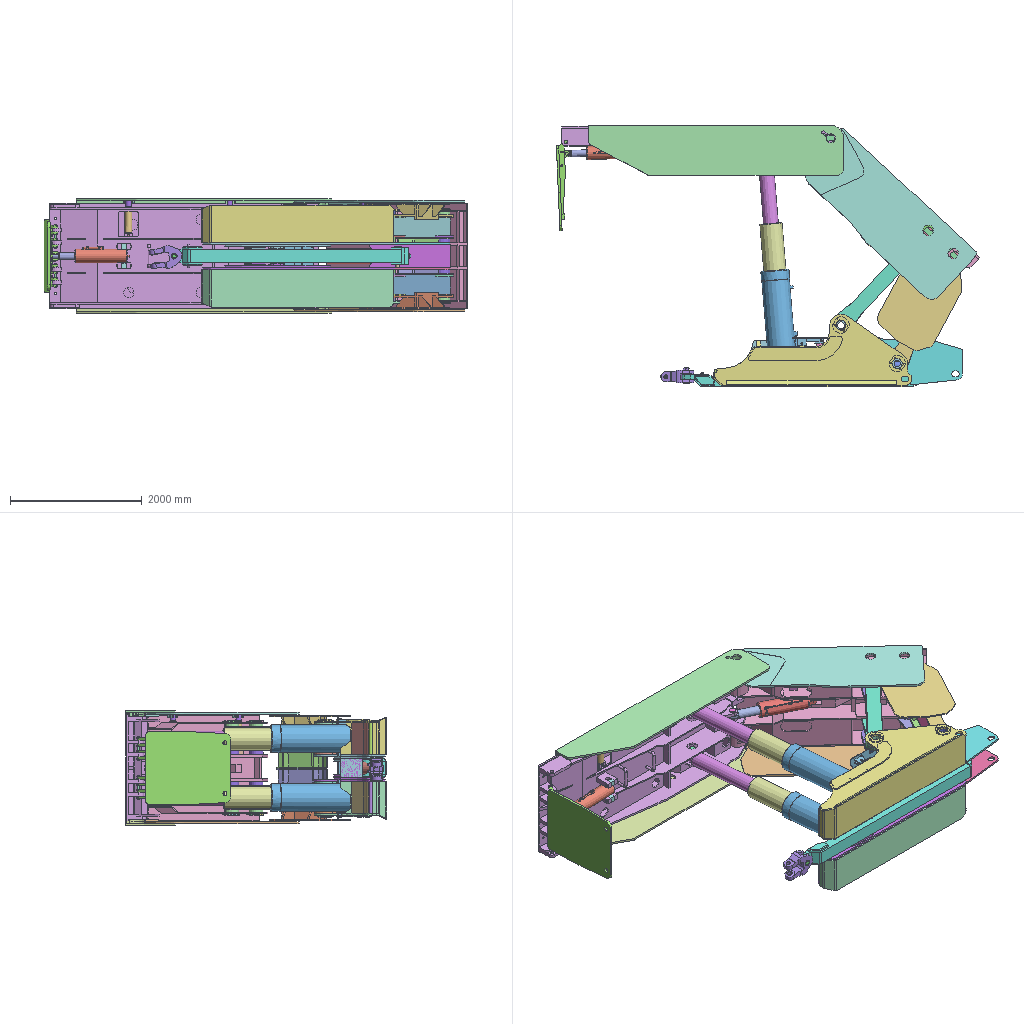Assembly | NX | 121 different items | 178 placed | box 6418 x 3966 x 1741 mm
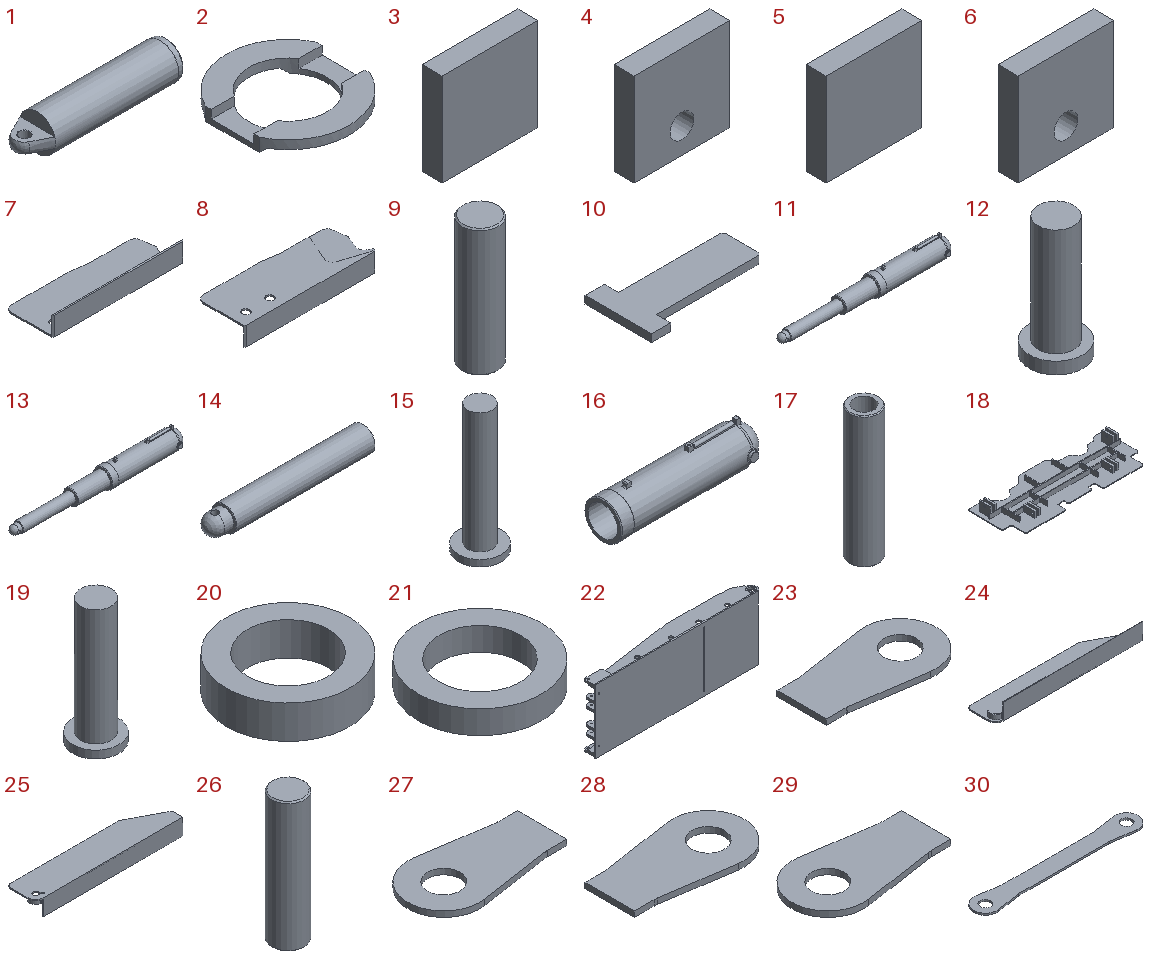Parts list (item | quantity | parent item | size | volume | features):
1 | x4 | in 56, 67, 78, 89 | 448 x 106 x 106 mm | 2799935 mm3 | features 侧推千斤顶缸 2
2 | x1 | in 34 | 207.123 x 230 x 25 mm | 362169 mm3 | features 掩护梁 2
3 | x1 | in 34 | 120 x 25 x 116 mm | 333863 mm3 | features 掩护梁 2
4 | x1 | in 34 | 120 x 25 x 116 mm | 330329 mm3 | features 掩护梁 2
5 | x1 | in 34 | 120 x 25 x 116 mm | 333863 mm3 | features 掩护梁 2
6 | x1 | in 34 | 120 x 25 x 116 mm | 330329 mm3 | features 掩护梁 2
7 | x1 | in 34 | 2828 x 1030 x 405 mm | 109386503 mm3 | features 掩护梁侧护板右 2
8 | x1 | in 34 | 2828 x 1030 x 405 mm | 109946345 mm3 | features 掩护梁侧护板左 2
9 | x4 | - | 145 x 145 x 511 mm | 8427015 mm3 | features 掩护梁连杆柱销 2
10 | x6 | in 34 | 260 x 140 x 16 mm | 370800 mm3 | features 梁销挡板 2
11 | x1 | - | 3742 x 478 x 474 mm | 232387520 mm3 | features 立柱活塞 2, 立柱缸一级 2, 立柱缸二级 2
12 | x4 | in 34 | 45 x 45 x 100 mm | 79522 mm3 | features 侧推千斤顶缸销 2
13 | x1 | - | 3742 x 478 x 474 mm | 232387520 mm3 | features 立柱活塞 2, 立柱缸一级 2, 立柱缸二级 2
14 | x2 | in 11, 13 | 1466 x 228.3 x 228.3 mm | 56225890 mm3 | features 立柱活塞 2
15 | x2 | - | 100 x 100 x 295 mm | 832302 mm3 | features 立柱活塞销 2
16 | x2 | in 11, 13 | 1697 x 478 x 474 mm | 93646895 mm3 | features 立柱缸一级 2
17 | x2 | in 11, 13 | 337.48 x 337.48 x 1508 mm | 82514797 mm3 | features 立柱缸二级 2
18 | x1 | in 45 | 1560 x 608.47 x 118 mm | 9927777 mm3 | features 脚踏板 2
19 | x4 | in 45 | 30 x 30 x 81 mm | 27410 mm3 | features 脚踏板柱销 2
20 | x4 | - | 220 x 220 x 59.435 mm | 1277869 mm3 | features 连杆套筒内 2
21 | x4 | - | 220 x 220 x 41.57 mm | 893766 mm3 | features 连杆套筒外 2
22 | x1 | in 34 | 4215 x 507.464 x 1600 mm | 647411376 mm3 | features 顶梁 2
23 | x2 | in 45 | 597.539 x 319.958 x 25 mm | 3444700 mm3 | features 前连杆 2
24 | x1 | in 34 | 3880 x 760 x 430 mm | 99045232 mm3 | features 顶梁侧护板右 2
25 | x1 | in 34 | 3880 x 760 x 430 mm | 99665785 mm3 | features 顶梁侧护板左 2
26 | x2 | in 34 | 130 x 130 x 520 mm | 6892131 mm3 | features 顶梁掩护板柱销 2
27 | x2 | in 45 | 597.539 x 319.958 x 25 mm | 3444700 mm3 | features 前连杆 2
28 | x2 | in 45 | 597.7 x 320 x 25 mm | 3443870 mm3 | features 前连杆 2
29 | x2 | in 45 | 597.7 x 320 x 25 mm | 3443870 mm3 | features 前连杆 2
30 | x2 | in 45 | 2260 x 320 x 25 mm | 12756678 mm3 | features 前连杆 2
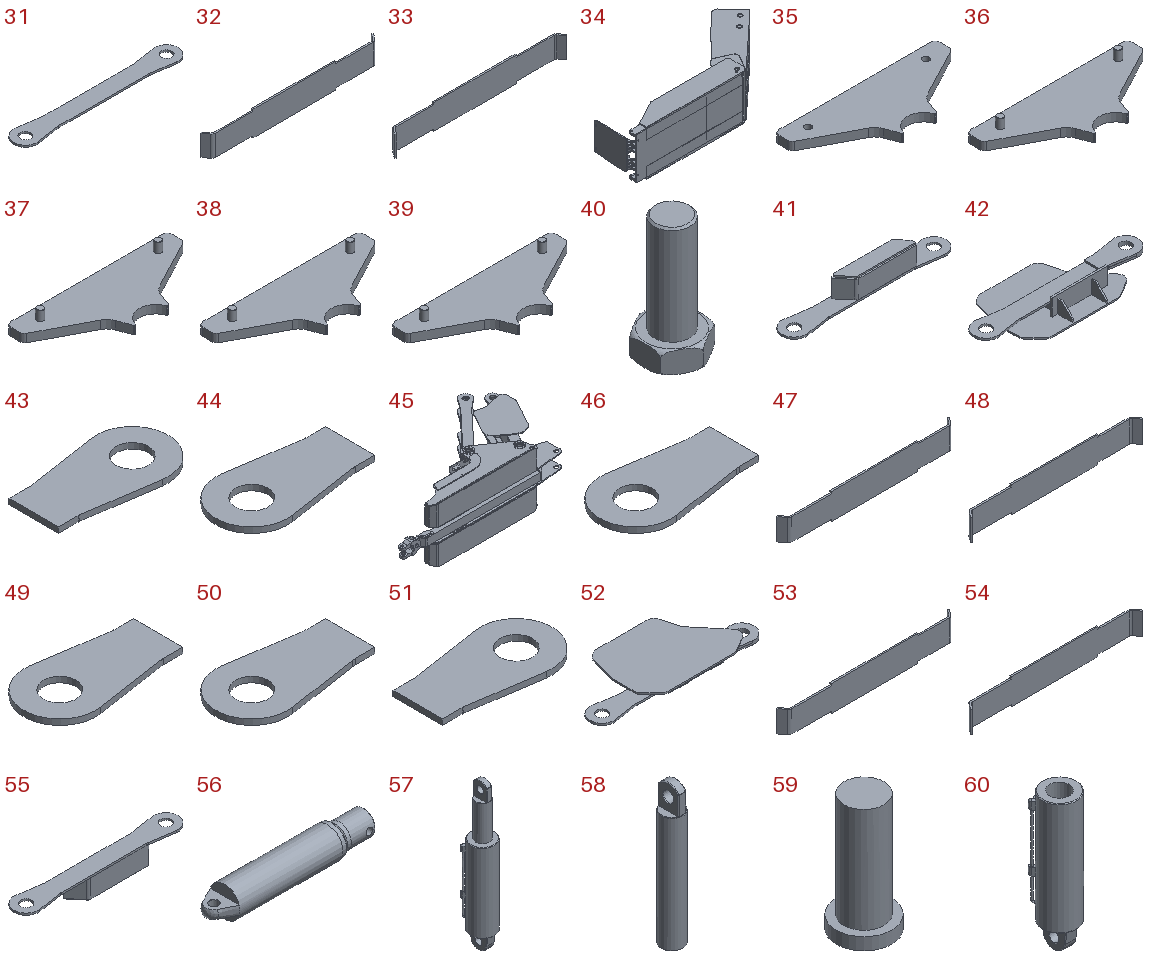31 | x2 | in 45 | 2260 x 320 x 25 mm | 12755026 mm3 | features 前连杆 2
32 | x2 | in 45 | 2216 x 103.15 x 320 mm | 12312626 mm3 | features 前连杆 2
33 | x2 | in 45 | 2216 x 103.15 x 320 mm | 12312626 mm3 | features 前连杆 2
34 | x1 | - | 6418 x 2642 x 1741 mm | 733546494 mm3 | features 掩护梁 16, 侧推千斤顶活塞 2, 侧推千斤顶活塞销 2, 侧推千斤顶缸 2, 侧推千斤顶缸销 2, 平衡千斤顶活塞 2, 平衡千斤顶活塞销 2, 平衡千斤顶缸 2, 平衡千斤顶缸销 2, 护帮千斤顶活塞 2, 护帮千斤顶缸 2, 护邦千斤顶活塞销 2, 护邦千斤顶滑块 2, 护邦千斤顶滑块销 2, 护邦销 2, 掩护梁侧护板右 2, 掩护梁侧护板左 2, 梁销挡板 2, 顶梁 2, 顶梁侧护板右 2, 顶梁侧护板左 2, 顶梁掩护板柱销 2
35 | x4 | in 36, 37, 38, 39 | 492 x 197.84 x 25 mm | 1447958 mm3 | features 压板 2
36 | x1 | - | 492 x 197.84 x 67 mm | 1501424 mm3 | features 压板 2, 压板螺钉 2
37 | x1 | - | 492 x 197.84 x 67 mm | 1501424 mm3 | features 压板 2, 压板螺钉 2
38 | x1 | - | 492 x 197.84 x 67 mm | 1501424 mm3 | features 压板 2, 压板螺钉 2
39 | x1 | - | 492 x 197.84 x 67 mm | 1501424 mm3 | features 压板 2, 压板螺钉 2
40 | x8 | in 36, 37, 38, 39 | 30.311 x 35 x 67 mm | 26733 mm3 | features 压板螺钉 2
41 | x1 | in 45 | 2165 x 320 x 280.474 mm | 23006049 mm3 | features 后连杆右 2
42 | x1 | in 45 | 2165 x 950 x 239.704 mm | 42809177 mm3 | features 后连杆右 2
43 | x1 | in 45 | 597.539 x 319.958 x 25 mm | 3444700 mm3 | features 后连杆右 2
44 | x1 | in 45 | 597.539 x 319.958 x 25 mm | 3444700 mm3 | features 后连杆右 2
45 | x1 | - | 4616 x 2509 x 1594 mm | 1068302240 mm3 | features 底座(默认<按焊接>) 68, 前连杆 16, 后连杆右 14, 后连杆左 14, 推移千斤顶活塞 2, 推移千斤顶约束块 2, 推移千斤顶约束销 2, 推移千斤顶缸 2, 推移杆 2, 推移杆柱销 2, 推移杆连接头 2, 推移杆连接头销柱 2, 脚踏板 2, 脚踏板柱销 2
46 | x1 | in 45 | 597.7 x 320 x 25 mm | 3443870 mm3 | features 后连杆右 2
47 | x1 | in 45 | 2121 x 103.15 x 320 mm | 11841435 mm3 | features 后连杆右 2
48 | x1 | in 45 | 2121 x 103.15 x 320 mm | 11841435 mm3 | features 后连杆右 2
49 | x1 | in 45 | 597.539 x 319.958 x 25 mm | 3444700 mm3 | features 后连杆左 2
50 | x1 | in 45 | 597.7 x 320 x 25 mm | 3443870 mm3 | features 后连杆左 2
51 | x1 | in 45 | 597.539 x 319.958 x 25 mm | 3444700 mm3 | features 后连杆左 2
52 | x1 | in 45 | 2165 x 950 x 239.704 mm | 42809177 mm3 | features 后连杆左 2
53 | x1 | in 45 | 2121 x 103.15 x 320 mm | 11841435 mm3 | features 后连杆左 2
54 | x1 | in 45 | 2121 x 103.15 x 320 mm | 11841435 mm3 | features 后连杆左 2
55 | x1 | in 45 | 2165 x 320 x 288.399 mm | 23380345 mm3 | features 后连杆左 2
56 | x1 | in 34 | 557.21 x 106 x 106 mm | 4001639 mm3 | features 侧推千斤顶活塞 2, 侧推千斤顶缸 2
57 | x1 | in 34 | 232.246 x 266.383 x 1421 mm | 35196422 mm3 | features 平衡千斤顶活塞 2, 平衡千斤顶缸 2
58 | x1 | in 57 | 135 x 135 x 882.27 mm | 11180627 mm3 | features 平衡千斤顶活塞 2
59 | x1 | in 34 | 90 x 90 x 190 mm | 691347 mm3 | features 平衡千斤顶活塞销 2
60 | x1 | in 57 | 232.246 x 266.383 x 924.565 mm | 24015479 mm3 | features 平衡千斤顶缸 2
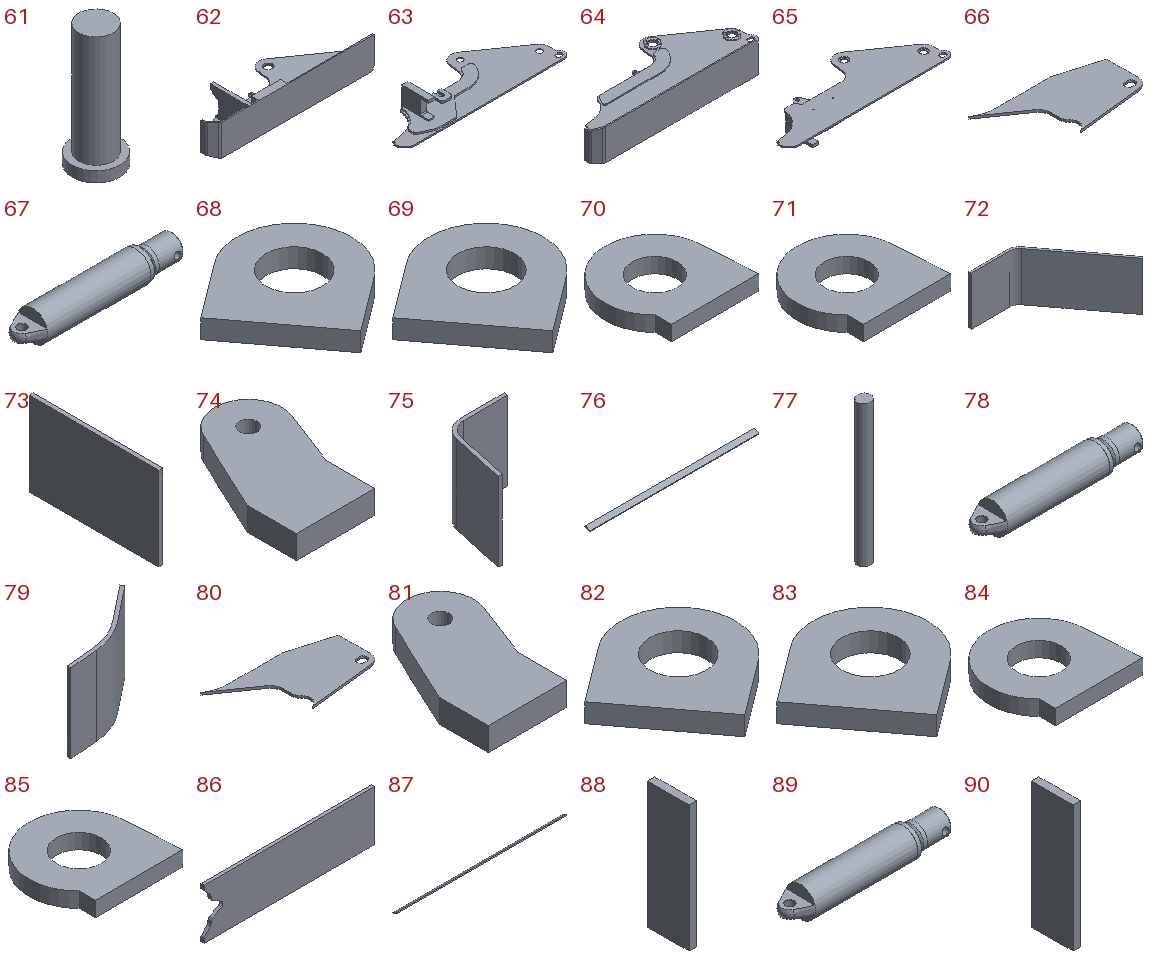61 | x1 | in 34 | 90 x 90 x 230 mm | 824079 mm3 | features 平衡千斤顶缸销 2
62 | x1 | in 45 | 3009 x 1102 x 567 mm | 135543302 mm3 | features 底座(默认<按焊接>) 2
63 | x1 | in 45 | 2987 x 1080 x 386 mm | 80381862 mm3 | features 底座(默认<按焊接>) 2
64 | x1 | in 45 | 3009 x 1102 x 567 mm | 135543302 mm3 | features 底座(默认<按焊接>) 2
65 | x1 | in 45 | 2987 x 1080 x 386 mm | 80381862 mm3 | features 底座(默认<按焊接>) 2
66 | x1 | in 45 | 1332 x 758.269 x 26 mm | 13979439 mm3 | features 底座(默认<按焊接>) 2
67 | x1 | in 34 | 557.21 x 106 x 106 mm | 4001639 mm3 | features 侧推千斤顶活塞 2, 侧推千斤顶缸 2
68 | x1 | in 45 | 381.454 x 376.184 x 50 mm | 3554006 mm3 | features 底座(默认<按焊接>) 2
69 | x1 | in 45 | 381.454 x 376.184 x 50 mm | 3554006 mm3 | features 底座(默认<按焊接>) 2
70 | x1 | in 45 | 339.407 x 334 x 50 mm | 3868356 mm3 | features 底座(默认<按焊接>) 2
71 | x1 | in 45 | 339.407 x 334 x 50 mm | 3868356 mm3 | features 底座(默认<按焊接>) 2
72 | x1 | in 45 | 988.426 x 741.88 x 480 mm | 13960123 mm3 | features 底座(默认<按焊接>) 2
73 | x1 | in 45 | 21.82 x 741.88 x 480 mm | 7770154 mm3 | features 底座(默认<按焊接>) 2
74 | x1 | in 45 | 113.6 x 167.23 x 26 mm | 337496 mm3 | features 底座(默认<按焊接>) 2
75 | x1 | in 45 | 457.703 x 425.5 x 480 mm | 7854055 mm3 | features 底座(默认<按焊接>) 2
76 | x1 | in 45 | 2570 x 74.293 x 53.683 mm | 3173441 mm3 | features 底座(默认<按焊接>) 2
77 | x1 | in 45 | 44.892 x 44.892 x 480 mm | 759747 mm3 | features 底座(默认<按焊接>) 2
78 | x1 | in 34 | 562.21 x 106 x 106 mm | 4001639 mm3 | features 侧推千斤顶活塞 2, 侧推千斤顶缸 2
79 | x1 | in 45 | 600.05 x 287.774 x 480 mm | 7044002 mm3 | features 底座(默认<按焊接>) 2
80 | x1 | in 45 | 1332 x 758.269 x 26 mm | 13979439 mm3 | features 底座(默认<按焊接>) 2
81 | x1 | in 45 | 113.6 x 167.23 x 26 mm | 337496 mm3 | features 底座(默认<按焊接>) 2
82 | x1 | in 45 | 381.454 x 376.184 x 50 mm | 3554006 mm3 | features 底座(默认<按焊接>) 2
83 | x1 | in 45 | 381.454 x 376.184 x 50 mm | 3554006 mm3 | features 底座(默认<按焊接>) 2
84 | x1 | in 45 | 339.407 x 334 x 50 mm | 3868356 mm3 | features 底座(默认<按焊接>) 2
85 | x1 | in 45 | 339.407 x 334 x 50 mm | 3868356 mm3 | features 底座(默认<按焊接>) 2
86 | x1 | in 45 | 1222 x 21.82 x 360 mm | 9202426 mm3 | features 底座(默认<按焊接>) 2
87 | x1 | in 45 | 2570 x 74.293 x 53.683 mm | 3173441 mm3 | features 底座(默认<按焊接>) 2
88 | x1 | in 45 | 20 x 116.68 x 360 mm | 840096 mm3 | features 底座(默认<按焊接>) 2
89 | x1 | in 34 | 562.21 x 106 x 106 mm | 4001639 mm3 | features 侧推千斤顶活塞 2, 侧推千斤顶缸 2
90 | x1 | in 45 | 20 x 116.68 x 360 mm | 840096 mm3 | features 底座(默认<按焊接>) 2
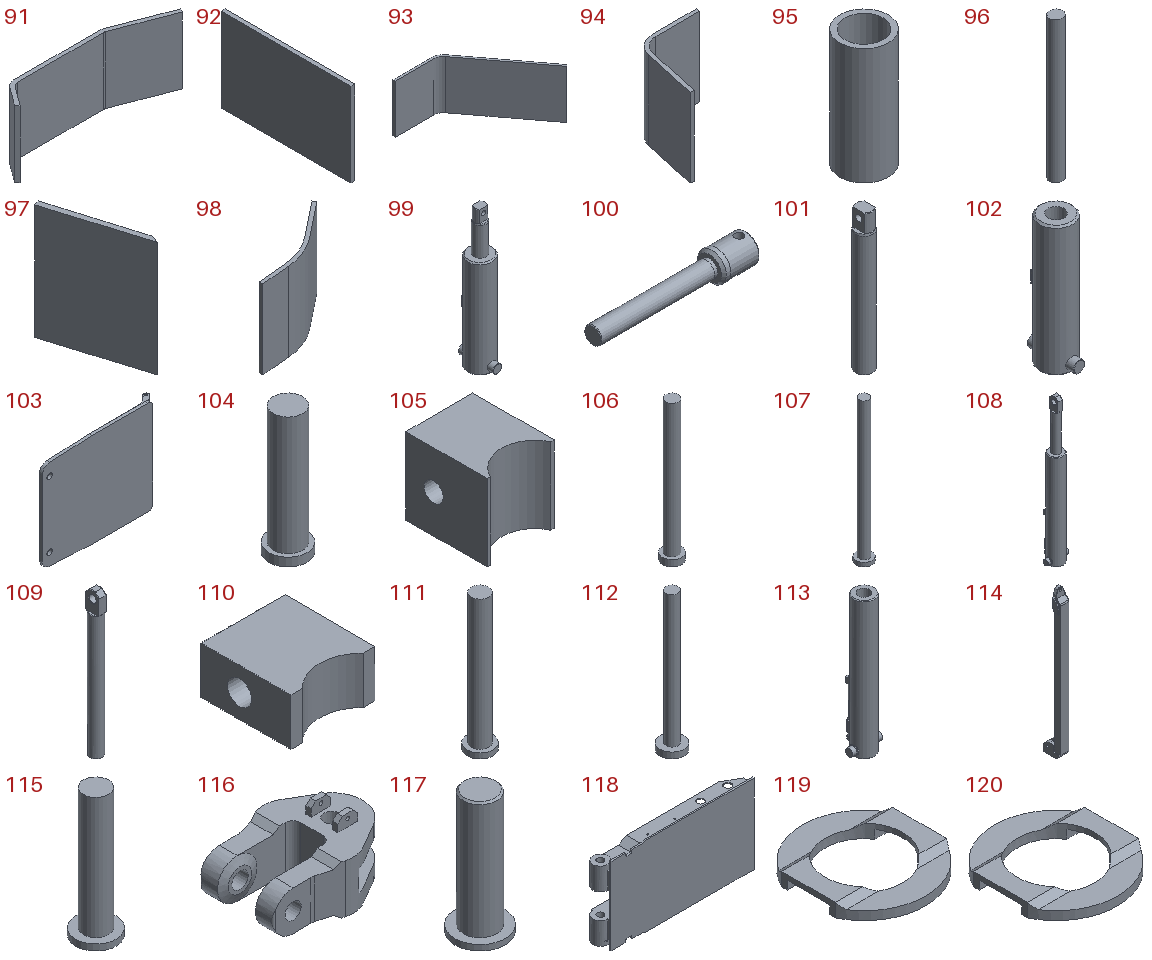91 | x1 | in 45 | 901.587 x 137.68 x 360 mm | 7322251 mm3 | features 底座(默认<按焊接>) 2
92 | x1 | in 45 | 21.82 x 741.88 x 480 mm | 7770154 mm3 | features 底座(默认<按焊接>) 2
93 | x1 | in 45 | 988.426 x 741.88 x 480 mm | 13960123 mm3 | features 底座(默认<按焊接>) 2
94 | x1 | in 45 | 457.703 x 425.5 x 480 mm | 7854055 mm3 | features 底座(默认<按焊接>) 2
95 | x1 | in 45 | 200.744 x 200.744 x 480 mm | 5887277 mm3 | features 底座(默认<按焊接>) 2
96 | x1 | in 45 | 44.892 x 44.892 x 480 mm | 759747 mm3 | features 底座(默认<按焊接>) 2
97 | x1 | in 45 | 133.231 x 399.146 x 480 mm | 4164554 mm3 | features 底座(默认<按焊接>) 2
98 | x1 | in 45 | 600.05 x 287.774 x 480 mm | 7044002 mm3 | features 底座(默认<按焊接>) 2
99 | x1 | in 34 | 203 x 287 x 1169 mm | 26817632 mm3 | features 护帮千斤顶活塞 2, 护帮千斤顶缸 2
100 | x4 | in 56, 67, 78, 89 | 449.94 x 84 x 84 mm | 1201706 mm3 | features 侧推千斤顶活塞 2
101 | x1 | in 99 | 100 x 100 x 798 mm | 5913177 mm3 | features 护帮千斤顶活塞 2
102 | x1 | in 99 | 203 x 287 x 828 mm | 20904449 mm3 | features 护帮千斤顶缸 2
103 | x1 | in 34 | - | - | features 护邦 2
104 | x1 | in 34 | 45 x 45 x 150 mm | 150600 mm3 | features 护邦千斤顶活塞销 2
105 | x2 | in 34 | 70 x 85 x 80 mm | 381423 mm3 | features 护邦千斤顶滑块 2
106 | x2 | in 34 | 30 x 30 x 220 mm | 73042 mm3 | features 护邦千斤顶滑块销 2
107 | x2 | in 34 | 40 x 40 x 360 mm | 184372 mm3 | features 护邦销 2
108 | x1 | in 45 | 287 x 247.6 x 1967 mm | 40401860 mm3 | features 推移千斤顶活塞 2, 推移千斤顶缸 2
109 | x1 | in 108 | 106.3 x 120.47 x 1261 mm | 10694769 mm3 | features 推移千斤顶活塞 2
110 | x2 | in 45 | 70 x 75 x 39.28 mm | 169219 mm3 | features 推移千斤顶约束块 2
111 | x4 | in 34 | 30 x 30 x 156 mm | 51365 mm3 | features 侧推千斤顶活塞销 2
112 | x2 | in 45 | 40 x 40 x 230 mm | 81681 mm3 | features 推移千斤顶约束销 2
113 | x1 | in 108 | 287 x 247.6 x 1299 mm | 29707096 mm3 | features 推移千斤顶缸 2
114 | x1 | in 45 | 283.14 x 415 x 3654 mm | 76372514 mm3 | features 推移杆 2
115 | x1 | in 45 | 100 x 100 x 315 mm | 1023531 mm3 | features 推移杆柱销 2
116 | x1 | in 45 | 486.5 x 347.5 x 233.365 mm | 11889729 mm3 | features 推移杆连接头 2
117 | x1 | in 45 | 90 x 90 x 220 mm | 656558 mm3 | features 推移杆连接头销柱 2
118 | x1 | in 34 | - | - | features 掩护梁 2
119 | x1 | in 34 | 207.123 x 230 x 25 mm | 366015 mm3 | features 掩护梁 2
120 | x1 | in 34 | 207.123 x 230 x 25 mm | 366015 mm3 | features 掩护梁 2
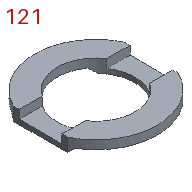121 | x1 | in 34 | 207.123 x 230 x 25 mm | 362169 mm3 | features 掩护梁 2